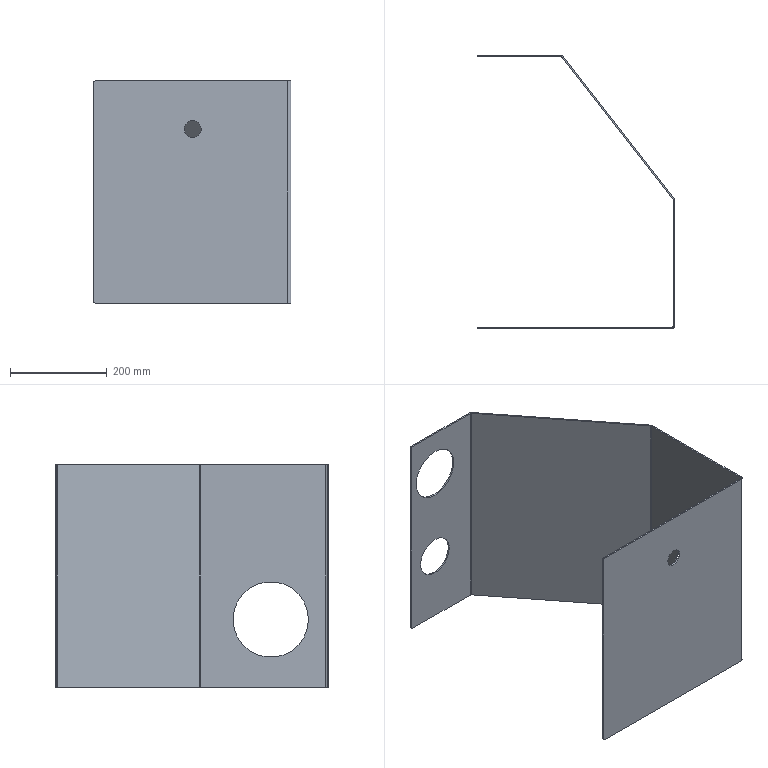Part | SolidWorks | features Cut 3, FlatPattern 1, ICE 1, SMBaseFlange 1, SheetMetal 1 | 1 solid | 42 faces | box 409 x 566 x 460 mm | volume 1582999 mm3 | plane 24 | cylinder 18 | commonest cylinder face diameters 10 x4 6 x3 12 x3 35 x2 84 x2 110 x2
STEP:
#1=CARTESIAN_POINT('',(67.,563.,305.));
#2=VERTEX_POINT('',#1);
#3=CARTESIAN_POINT('',(67.,563.,415.));
#4=VERTEX_POINT('',#3);
#5=CARTESIAN_POINT('',(67.,563.,360.));
#6=DIRECTION('',(0.,1.,0.));
#7=DIRECTION('',(0.,0.,1.));
#8=AXIS2_PLACEMENT_3D('',#5,#6,#7);
#9=CIRCLE('',#8,55.);
#10=EDGE_CURVE('',#2,#4,#9,.T.);
#11=ORIENTED_EDGE('',*,*,#10,.F.);
#12=CARTESIAN_POINT('',(67.,566.,305.));
#13=VERTEX_POINT('',#12);
#14=CARTESIAN_POINT('',(67.,563.,305.));
#15=DIRECTION('',(0.,1.,0.));
#16=VECTOR('',#15,1000.);
#17=LINE('',#14,#16);
#18=EDGE_CURVE('',#2,#13,#17,.T.);
#19=ORIENTED_EDGE('',*,*,#18,.T.);
#20=CARTESIAN_POINT('',(67.,566.,415.));
#21=VERTEX_POINT('',#20);
#22=CARTESIAN_POINT('',(67.,566.,360.));
#23=DIRECTION('',(0.,1.,0.));
#24=DIRECTION('',(0.,0.,1.));
#25=AXIS2_PLACEMENT_3D('',#22,#23,#24);
#26=CIRCLE('',#25,55.);
#27=EDGE_CURVE('',#13,#21,#26,.T.);
#28=ORIENTED_EDGE('',*,*,#27,.T.);
#29=CARTESIAN_POINT('',(67.,563.,415.));
#30=DIRECTION('',(0.,1.,0.));
#31=VECTOR('',#30,1000.);
#32=LINE('',#29,#31);
#33=EDGE_CURVE('',#4,#21,#32,.T.);
#34=ORIENTED_EDGE('',*,*,#33,.F.);
#35=EDGE_LOOP('',(#11,#19,#28,#34));
#36=FACE_OUTER_BOUND('',#35,.T.);
#37=CARTESIAN_POINT('',(67.,563.,360.));
#38=DIRECTION('',(0.,1.,0.));
#39=DIRECTION('',(0.,0.,1.));
#40=AXIS2_PLACEMENT_3D('',#37,#38,#39);
#41=CYLINDRICAL_SURFACE('',#40,55.);
#42=ADVANCED_FACE('',(#36),#41,.F.);
#43=CARTESIAN_POINT('',(67.,563.,108.));
#44=VERTEX_POINT('',#43);
#45=CARTESIAN_POINT('',(67.,563.,192.));
#46=VERTEX_POINT('',#45);
#47=CARTESIAN_POINT('',(67.,563.,150.));
#48=DIRECTION('',(0.,1.,0.));
#49=DIRECTION('',(0.,0.,1.));
#50=AXIS2_PLACEMENT_3D('',#47,#48,#49);
#51=CIRCLE('',#50,42.);
#52=EDGE_CURVE('',#44,#46,#51,.T.);
#53=ORIENTED_EDGE('',*,*,#52,.F.);
#54=CARTESIAN_POINT('',(67.,566.,108.));
#55=VERTEX_POINT('',#54);
#56=CARTESIAN_POINT('',(67.,563.,108.));
#57=DIRECTION('',(0.,1.,0.));
#58=VECTOR('',#57,1000.);
#59=LINE('',#56,#58);
#60=EDGE_CURVE('',#44,#55,#59,.T.);
#61=ORIENTED_EDGE('',*,*,#60,.T.);
#62=CARTESIAN_POINT('',(67.,566.,192.));
#63=VERTEX_POINT('',#62);
#64=CARTESIAN_POINT('',(67.,566.,150.));
#65=DIRECTION('',(0.,1.,0.));
#66=DIRECTION('',(0.,0.,1.));
#67=AXIS2_PLACEMENT_3D('',#64,#65,#66);
#68=CIRCLE('',#67,42.);
#69=EDGE_CURVE('',#55,#63,#68,.T.);
#70=ORIENTED_EDGE('',*,*,#69,.T.);
#71=CARTESIAN_POINT('',(67.,563.,192.));
#72=DIRECTION('',(0.,1.,0.));
#73=VECTOR('',#72,1000.);
#74=LINE('',#71,#73);
#75=EDGE_CURVE('',#46,#63,#74,.T.);
#76=ORIENTED_EDGE('',*,*,#75,.F.);
#77=EDGE_LOOP('',(#53,#61,#70,#76));
#78=FACE_OUTER_BOUND('',#77,.T.);
#79=CARTESIAN_POINT('',(67.,563.,150.));
#80=DIRECTION('',(0.,1.,0.));
#81=DIRECTION('',(0.,0.,1.));
#82=AXIS2_PLACEMENT_3D('',#79,#80,#81);
#83=CYLINDRICAL_SURFACE('',#82,42.);
#84=ADVANCED_FACE('',(#78),#83,.F.);
#85=CARTESIAN_POINT('',(203.,3.,377.5));
#86=VERTEX_POINT('',#85);
#87=CARTESIAN_POINT('',(203.,3.,342.5));
#88=VERTEX_POINT('',#87);
#89=CARTESIAN_POINT('',(203.,3.,360.));
#90=DIRECTION('',(0.,-1.,0.));
#91=DIRECTION('',(0.,0.,-1.));
#92=AXIS2_PLACEMENT_3D('',#89,#90,#91);
#93=CIRCLE('',#92,17.5);
#94=EDGE_CURVE('',#86,#88,#93,.T.);
#95=ORIENTED_EDGE('',*,*,#94,.F.);
#96=CARTESIAN_POINT('',(203.,0.,377.5));
#97=VERTEX_POINT('',#96);
#98=CARTESIAN_POINT('',(203.,3.,377.5));
#99=DIRECTION('',(0.,-1.,0.));
#100=VECTOR('',#99,1000.);
#101=LINE('',#98,#100);
#102=EDGE_CURVE('',#86,#97,#101,.T.);
#103=ORIENTED_EDGE('',*,*,#102,.T.);
#104=CARTESIAN_POINT('',(203.,0.,342.5));
#105=VERTEX_POINT('',#104);
#106=CARTESIAN_POINT('',(203.,0.,360.));
#107=DIRECTION('',(0.,-1.,0.));
#108=DIRECTION('',(0.,0.,-1.));
#109=AXIS2_PLACEMENT_3D('',#106,#107,#108);
#110=CIRCLE('',#109,17.5);
#111=EDGE_CURVE('',#97,#105,#110,.T.);
#112=ORIENTED_EDGE('',*,*,#111,.T.);
#113=CARTESIAN_POINT('',(203.,3.,342.5));
#114=DIRECTION('',(0.,-1.,0.));
#115=VECTOR('',#114,1000.);
#116=LINE('',#113,#115);
#117=EDGE_CURVE('',#88,#105,#116,.T.);
#118=ORIENTED_EDGE('',*,*,#117,.F.);
#119=EDGE_LOOP('',(#95,#103,#112,#118));
#120=FACE_OUTER_BOUND('',#119,.T.);
#121=CARTESIAN_POINT('',(203.,3.,360.));
#122=DIRECTION('',(0.,-1.,0.));
#123=DIRECTION('',(0.,0.,-1.));
#124=AXIS2_PLACEMENT_3D('',#121,#122,#123);
#125=CYLINDRICAL_SURFACE('',#124,17.5);
#126=ADVANCED_FACE('',(#120),#125,.F.);
#127=CARTESIAN_POINT('',(403.,42.,140.));
#128=VERTEX_POINT('',#127);
#129=CARTESIAN_POINT('',(403.,198.,140.));
#130=VERTEX_POINT('',#129);
#131=CARTESIAN_POINT('',(403.,120.,140.));
#132=DIRECTION('',(1.,0.,0.));
#133=DIRECTION('',(0.,1.,0.));
#134=AXIS2_PLACEMENT_3D('',#131,#132,#133);
#135=CIRCLE('',#134,78.);
#136=EDGE_CURVE('',#128,#130,#135,.T.);
#137=ORIENTED_EDGE('',*,*,#136,.F.);
#138=CARTESIAN_POINT('',(406.,42.,140.));
#139=VERTEX_POINT('',#138);
#140=CARTESIAN_POINT('',(396.,42.,140.));
#141=DIRECTION('',(1.,0.,0.));
#142=VECTOR('',#141,1000.);
#143=LINE('',#140,#142);
#144=EDGE_CURVE('',#128,#139,#143,.T.);
#145=ORIENTED_EDGE('',*,*,#144,.T.);
#146=CARTESIAN_POINT('',(406.,198.,140.));
#147=VERTEX_POINT('',#146);
#148=CARTESIAN_POINT('',(406.,120.,140.));
#149=DIRECTION('',(1.,0.,0.));
#150=DIRECTION('',(0.,1.,0.));
#151=AXIS2_PLACEMENT_3D('',#148,#149,#150);
#152=CIRCLE('',#151,78.);
#153=EDGE_CURVE('',#139,#147,#152,.T.);
#154=ORIENTED_EDGE('',*,*,#153,.T.);
#155=CARTESIAN_POINT('',(396.,198.,140.));
#156=DIRECTION('',(1.,0.,0.));
#157=VECTOR('',#156,1000.);
#158=LINE('',#155,#157);
#159=EDGE_CURVE('',#130,#147,#158,.T.);
#160=ORIENTED_EDGE('',*,*,#159,.F.);
#161=EDGE_LOOP('',(#137,#145,#154,#160));
#162=FACE_OUTER_BOUND('',#161,.T.);
#163=CARTESIAN_POINT('',(396.,120.,140.));
#164=DIRECTION('',(1.,0.,0.));
#165=DIRECTION('',(0.,1.,0.));
#166=AXIS2_PLACEMENT_3D('',#163,#164,#165);
#167=CYLINDRICAL_SURFACE('',#166,78.);
#168=ADVANCED_FACE('',(#162),#167,.F.);
#169=CARTESIAN_POINT('',(67.,566.,360.));
#170=DIRECTION('',(0.,1.,0.));
#171=DIRECTION('',(0.,0.,1.));
#172=AXIS2_PLACEMENT_3D('',#169,#170,#171);
#173=CIRCLE('',#172,55.);
#174=EDGE_CURVE('',#21,#13,#173,.T.);
#175=ORIENTED_EDGE('',*,*,#174,.F.);
#176=ORIENTED_EDGE('',*,*,#27,.F.);
#177=EDGE_LOOP('',(#175,#176));
#178=FACE_BOUND('',#177,.T.);
#179=CARTESIAN_POINT('',(67.,566.,150.));
#180=DIRECTION('',(0.,1.,0.));
#181=DIRECTION('',(0.,0.,1.));
#182=AXIS2_PLACEMENT_3D('',#179,#180,#181);
#183=CIRCLE('',#182,42.);
#184=EDGE_CURVE('',#63,#55,#183,.T.);
#185=ORIENTED_EDGE('',*,*,#184,.F.);
#186=ORIENTED_EDGE('',*,*,#69,.F.);
#187=EDGE_LOOP('',(#185,#186));
#188=FACE_BOUND('',#187,.T.);
#189=CARTESIAN_POINT('',(2.,566.,0.));
#190=VERTEX_POINT('',#189);
#191=CARTESIAN_POINT('',(170.25,566.,0.));
#192=VERTEX_POINT('',#191);
#193=CARTESIAN_POINT('',(-3.,566.,0.));
#194=DIRECTION('',(1.,0.,0.));
#195=VECTOR('',#194,1000.);
#196=LINE('',#193,#195);
#197=EDGE_CURVE('',#190,#192,#196,.T.);
#198=ORIENTED_EDGE('',*,*,#197,.F.);
#199=CARTESIAN_POINT('',(-3.,566.,5.));
#200=VERTEX_POINT('',#199);
#201=CARTESIAN_POINT('',(2.,566.,5.));
#202=DIRECTION('',(0.,-1.,0.));
#203=DIRECTION('',(0.,0.,1.));
#204=AXIS2_PLACEMENT_3D('',#201,#202,#203);
#205=CIRCLE('',#204,5.);
#206=EDGE_CURVE('',#200,#190,#205,.T.);
#207=ORIENTED_EDGE('',*,*,#206,.F.);
#208=CARTESIAN_POINT('',(-3.,566.,455.));
#209=VERTEX_POINT('',#208);
#210=CARTESIAN_POINT('',(-3.,566.,460.));
#211=DIRECTION('',(0.,0.,-1.));
#212=VECTOR('',#211,1000.);
#213=LINE('',#210,#212);
#214=EDGE_CURVE('',#209,#200,#213,.T.);
#215=ORIENTED_EDGE('',*,*,#214,.F.);
#216=CARTESIAN_POINT('',(2.,566.,460.));
#217=VERTEX_POINT('',#216);
#218=CARTESIAN_POINT('',(2.,566.,455.));
#219=DIRECTION('',(0.,-1.,0.));
#220=DIRECTION('',(0.,0.,1.));
#221=AXIS2_PLACEMENT_3D('',#218,#219,#220);
#222=CIRCLE('',#221,5.);
#223=EDGE_CURVE('',#217,#209,#222,.T.);
#224=ORIENTED_EDGE('',*,*,#223,.F.);
#225=CARTESIAN_POINT('',(170.25,566.,460.));
#226=VERTEX_POINT('',#225);
#227=CARTESIAN_POINT('',(-3.,566.,460.));
#228=DIRECTION('',(1.,0.,0.));
#229=VECTOR('',#228,1000.);
#230=LINE('',#227,#229);
#231=EDGE_CURVE('',#217,#226,#230,.T.);
#232=ORIENTED_EDGE('',*,*,#231,.T.);
#233=CARTESIAN_POINT('',(170.25,566.,460.));
#234=DIRECTION('',(0.,0.,-1.));
#235=VECTOR('',#234,1000.);
#236=LINE('',#233,#235);
#237=EDGE_CURVE('',#226,#192,#236,.T.);
#238=ORIENTED_EDGE('',*,*,#237,.T.);
#239=EDGE_LOOP('',(#198,#207,#215,#224,#232,#238));
#240=FACE_OUTER_BOUND('',#239,.T.);
#241=CARTESIAN_POINT('',(-3.,566.,460.));
#242=DIRECTION('',(0.,1.,0.));
#243=DIRECTION('',(0.,0.,1.));
#244=AXIS2_PLACEMENT_3D('',#241,#242,#243);
#245=PLANE('',#244);
#246=ADVANCED_FACE('',(#178,#188,#240),#245,.T.);
#247=CARTESIAN_POINT('',(67.,563.,360.));
#248=DIRECTION('',(0.,1.,0.));
#249=DIRECTION('',(0.,0.,1.));
#250=AXIS2_PLACEMENT_3D('',#247,#248,#249);
#251=CIRCLE('',#250,55.);
#252=EDGE_CURVE('',#4,#2,#251,.T.);
#253=ORIENTED_EDGE('',*,*,#252,.T.);
#254=ORIENTED_EDGE('',*,*,#10,.T.);
#255=EDGE_LOOP('',(#253,#254));
#256=FACE_BOUND('',#255,.T.);
#257=CARTESIAN_POINT('',(67.,563.,150.));
#258=DIRECTION('',(0.,1.,0.));
#259=DIRECTION('',(0.,0.,1.));
#260=AXIS2_PLACEMENT_3D('',#257,#258,#259);
#261=CIRCLE('',#260,42.);
#262=EDGE_CURVE('',#46,#44,#261,.T.);
#263=ORIENTED_EDGE('',*,*,#262,.T.);
#264=ORIENTED_EDGE('',*,*,#52,.T.);
#265=EDGE_LOOP('',(#263,#264));
#266=FACE_BOUND('',#265,.T.);
#267=CARTESIAN_POINT('',(-3.,563.,5.));
#268=VERTEX_POINT('',#267);
#269=CARTESIAN_POINT('',(2.,563.,0.));
#270=VERTEX_POINT('',#269);
#271=CARTESIAN_POINT('',(2.,563.,5.));
#272=DIRECTION('',(0.,-1.,0.));
#273=DIRECTION('',(0.,0.,1.));
#274=AXIS2_PLACEMENT_3D('',#271,#272,#273);
#275=CIRCLE('',#274,5.);
#276=EDGE_CURVE('',#268,#270,#275,.T.);
#277=ORIENTED_EDGE('',*,*,#276,.T.);
#278=CARTESIAN_POINT('',(170.25,563.,0.));
#279=VERTEX_POINT('',#278);
#280=CARTESIAN_POINT('',(-3.,563.,0.));
#281=DIRECTION('',(1.,0.,0.));
#282=VECTOR('',#281,1000.);
#283=LINE('',#280,#282);
#284=EDGE_CURVE('',#270,#279,#283,.T.);
#285=ORIENTED_EDGE('',*,*,#284,.T.);
#286=CARTESIAN_POINT('',(170.25,563.,460.));
#287=VERTEX_POINT('',#286);
#288=CARTESIAN_POINT('',(170.25,563.,460.));
#289=DIRECTION('',(0.,0.,-1.));
#290=VECTOR('',#289,1000.);
#291=LINE('',#288,#290);
#292=EDGE_CURVE('',#287,#279,#291,.T.);
#293=ORIENTED_EDGE('',*,*,#292,.F.);
#294=CARTESIAN_POINT('',(2.,563.,460.));
#295=VERTEX_POINT('',#294);
#296=CARTESIAN_POINT('',(-3.,563.,460.));
#297=DIRECTION('',(1.,0.,0.));
#298=VECTOR('',#297,1000.);
#299=LINE('',#296,#298);
#300=EDGE_CURVE('',#295,#287,#299,.T.);
#301=ORIENTED_EDGE('',*,*,#300,.F.);
#302=CARTESIAN_POINT('',(-3.,563.,455.));
#303=VERTEX_POINT('',#302);
#304=CARTESIAN_POINT('',(2.,563.,455.));
#305=DIRECTION('',(0.,-1.,0.));
#306=DIRECTION('',(0.,0.,1.));
#307=AXIS2_PLACEMENT_3D('',#304,#305,#306);
#308=CIRCLE('',#307,5.);
#309=EDGE_CURVE('',#295,#303,#308,.T.);
#310=ORIENTED_EDGE('',*,*,#309,.T.);
#311=CARTESIAN_POINT('',(-3.,563.,460.));
#312=DIRECTION('',(0.,0.,-1.));
#313=VECTOR('',#312,1000.);
#314=LINE('',#311,#313);
#315=EDGE_CURVE('',#303,#268,#314,.T.);
#316=ORIENTED_EDGE('',*,*,#315,.T.);
#317=EDGE_LOOP('',(#277,#285,#293,#301,#310,#316));
#318=FACE_OUTER_BOUND('',#317,.T.);
#319=CARTESIAN_POINT('',(-3.,563.,460.));
#320=DIRECTION('',(0.,1.,0.));
#321=DIRECTION('',(0.,0.,1.));
#322=AXIS2_PLACEMENT_3D('',#319,#320,#321);
#323=PLANE('',#322);
#324=ADVANCED_FACE('',(#256,#266,#318),#323,.F.);
#325=ORIENTED_EDGE('',*,*,#284,.F.);
#326=CARTESIAN_POINT('',(2.,563.,0.));
#327=DIRECTION('',(0.,1.,0.));
#328=VECTOR('',#327,1000.);
#329=LINE('',#326,#328);
#330=EDGE_CURVE('',#270,#190,#329,.T.);
#331=ORIENTED_EDGE('',*,*,#330,.T.);
#332=ORIENTED_EDGE('',*,*,#197,.T.);
#333=CARTESIAN_POINT('',(170.25,566.,0.));
#334=DIRECTION('',(0.,-1.,0.));
#335=VECTOR('',#334,1000.);
#336=LINE('',#333,#335);
#337=EDGE_CURVE('',#192,#279,#336,.T.);
#338=ORIENTED_EDGE('',*,*,#337,.T.);
#339=EDGE_LOOP('',(#325,#331,#332,#338));
#340=FACE_OUTER_BOUND('',#339,.T.);
#341=CARTESIAN_POINT('',(172.615,561.847,0.));
#342=DIRECTION('',(0.,0.,-1.));
#343=DIRECTION('',(-1.,0.,0.));
#344=AXIS2_PLACEMENT_3D('',#341,#342,#343);
#345=PLANE('',#344);
#346=ADVANCED_FACE('',(#340),#345,.T.);
#347=CARTESIAN_POINT('',(203.,0.,360.));
#348=DIRECTION('',(0.,-1.,0.));
#349=DIRECTION('',(0.,0.,-1.));
#350=AXIS2_PLACEMENT_3D('',#347,#348,#349);
#351=CIRCLE('',#350,17.5);
#352=EDGE_CURVE('',#105,#97,#351,.T.);
#353=ORIENTED_EDGE('',*,*,#352,.F.);
#354=ORIENTED_EDGE('',*,*,#111,.F.);
#355=EDGE_LOOP('',(#353,#354));
#356=FACE_BOUND('',#355,.T.);
#357=CARTESIAN_POINT('',(-3.,0.,455.));
#358=VERTEX_POINT('',#357);
#359=CARTESIAN_POINT('',(-3.,0.,5.));
#360=VERTEX_POINT('',#359);
#361=CARTESIAN_POINT('',(-3.,0.,460.));
#362=DIRECTION('',(0.,0.,-1.));
#363=VECTOR('',#362,1000.);
#364=LINE('',#361,#363);
#365=EDGE_CURVE('',#358,#360,#364,.T.);
#366=ORIENTED_EDGE('',*,*,#365,.T.);
#367=CARTESIAN_POINT('',(2.,0.,0.));
#368=VERTEX_POINT('',#367);
#369=CARTESIAN_POINT('',(2.,0.,5.));
#370=DIRECTION('',(0.,1.,0.));
#371=DIRECTION('',(0.,0.,-1.));
#372=AXIS2_PLACEMENT_3D('',#369,#370,#371);
#373=CIRCLE('',#372,5.);
#374=EDGE_CURVE('',#368,#360,#373,.T.);
#375=ORIENTED_EDGE('',*,*,#374,.F.);
#376=CARTESIAN_POINT('',(400.,0.,0.));
#377=VERTEX_POINT('',#376);
#378=CARTESIAN_POINT('',(0.,0.,0.));
#379=DIRECTION('',(-1.,0.,0.));
#380=VECTOR('',#379,1000.);
#381=LINE('',#378,#380);
#382=EDGE_CURVE('',#377,#368,#381,.T.);
#383=ORIENTED_EDGE('',*,*,#382,.F.);
#384=CARTESIAN_POINT('',(400.,0.,460.));
#385=VERTEX_POINT('',#384);
#386=CARTESIAN_POINT('',(400.,0.,460.));
#387=DIRECTION('',(0.,0.,-1.));
#388=VECTOR('',#387,1000.);
#389=LINE('',#386,#388);
#390=EDGE_CURVE('',#385,#377,#389,.T.);
#391=ORIENTED_EDGE('',*,*,#390,.F.);
#392=CARTESIAN_POINT('',(2.,0.,460.));
#393=VERTEX_POINT('',#392);
#394=CARTESIAN_POINT('',(0.,0.,460.));
#395=DIRECTION('',(-1.,0.,0.));
#396=VECTOR('',#395,1000.);
#397=LINE('',#394,#396);
#398=EDGE_CURVE('',#385,#393,#397,.T.);
#399=ORIENTED_EDGE('',*,*,#398,.T.);
#400=CARTESIAN_POINT('',(2.,0.,455.));
#401=DIRECTION('',(0.,1.,0.));
#402=DIRECTION('',(0.,0.,-1.));
#403=AXIS2_PLACEMENT_3D('',#400,#401,#402);
#404=CIRCLE('',#403,5.);
#405=EDGE_CURVE('',#358,#393,#404,.T.);
#406=ORIENTED_EDGE('',*,*,#405,.F.);
#407=EDGE_LOOP('',(#366,#375,#383,#391,#399,#406));
#408=FACE_OUTER_BOUND('',#407,.T.);
#409=CARTESIAN_POINT('',(0.,0.,460.));
#410=DIRECTION('',(0.,-1.,0.));
#411=DIRECTION('',(0.,0.,-1.));
#412=AXIS2_PLACEMENT_3D('',#409,#410,#411);
#413=PLANE('',#412);
#414=ADVANCED_FACE('',(#356,#408),#413,.T.);
#415=CARTESIAN_POINT('',(203.,3.,360.));
#416=DIRECTION('',(0.,-1.,0.));
#417=DIRECTION('',(0.,0.,-1.));
#418=AXIS2_PLACEMENT_3D('',#415,#416,#417);
#419=CIRCLE('',#418,17.5);
#420=EDGE_CURVE('',#88,#86,#419,.T.);
#421=ORIENTED_EDGE('',*,*,#420,.T.);
#422=ORIENTED_EDGE('',*,*,#94,.T.);
#423=EDGE_LOOP('',(#421,#422));
#424=FACE_BOUND('',#423,.T.);
#425=CARTESIAN_POINT('',(2.,3.,0.));
#426=VERTEX_POINT('',#425);
#427=CARTESIAN_POINT('',(-3.,3.,5.));
#428=VERTEX_POINT('',#427);
#429=CARTESIAN_POINT('',(2.,3.,5.));
#430=DIRECTION('',(0.,1.,0.));
#431=DIRECTION('',(0.,0.,-1.));
#432=AXIS2_PLACEMENT_3D('',#429,#430,#431);
#433=CIRCLE('',#432,5.);
#434=EDGE_CURVE('',#426,#428,#433,.T.);
#435=ORIENTED_EDGE('',*,*,#434,.T.);
#436=CARTESIAN_POINT('',(-3.,3.,455.));
#437=VERTEX_POINT('',#436);
#438=CARTESIAN_POINT('',(-3.,3.,460.));
#439=DIRECTION('',(0.,0.,-1.));
#440=VECTOR('',#439,1000.);
#441=LINE('',#438,#440);
#442=EDGE_CURVE('',#437,#428,#441,.T.);
#443=ORIENTED_EDGE('',*,*,#442,.F.);
#444=CARTESIAN_POINT('',(2.,3.,460.));
#445=VERTEX_POINT('',#444);
#446=CARTESIAN_POINT('',(2.,3.,455.));
#447=DIRECTION('',(0.,1.,0.));
#448=DIRECTION('',(0.,0.,-1.));
#449=AXIS2_PLACEMENT_3D('',#446,#447,#448);
#450=CIRCLE('',#449,5.);
#451=EDGE_CURVE('',#437,#445,#450,.T.);
#452=ORIENTED_EDGE('',*,*,#451,.T.);
#453=CARTESIAN_POINT('',(400.,3.,460.));
#454=VERTEX_POINT('',#453);
#455=CARTESIAN_POINT('',(0.,3.,460.));
#456=DIRECTION('',(-1.,0.,0.));
#457=VECTOR('',#456,1000.);
#458=LINE('',#455,#457);
#459=EDGE_CURVE('',#454,#445,#458,.T.);
#460=ORIENTED_EDGE('',*,*,#459,.F.);
#461=CARTESIAN_POINT('',(400.,3.,0.));
#462=VERTEX_POINT('',#461);
#463=CARTESIAN_POINT('',(400.,3.,460.));
#464=DIRECTION('',(0.,0.,-1.));
#465=VECTOR('',#464,1000.);
#466=LINE('',#463,#465);
#467=EDGE_CURVE('',#454,#462,#466,.T.);
#468=ORIENTED_EDGE('',*,*,#467,.T.);
#469=CARTESIAN_POINT('',(0.,3.,0.));
#470=DIRECTION('',(-1.,0.,0.));
#471=VECTOR('',#470,1000.);
#472=LINE('',#469,#471);
#473=EDGE_CURVE('',#462,#426,#472,.T.);
#474=ORIENTED_EDGE('',*,*,#473,.T.);
#475=EDGE_LOOP('',(#435,#443,#452,#460,#468,#474));
#476=FACE_OUTER_BOUND('',#475,.T.);
#477=CARTESIAN_POINT('',(0.,3.,460.));
#478=DIRECTION('',(0.,-1.,0.));
#479=DIRECTION('',(0.,0.,-1.));
#480=AXIS2_PLACEMENT_3D('',#477,#478,#479);
#481=PLANE('',#480);
#482=ADVANCED_FACE('',(#424,#476),#481,.F.);
#483=ORIENTED_EDGE('',*,*,#442,.T.);
#484=CARTESIAN_POINT('',(-3.,3.,5.));
#485=DIRECTION('',(0.,-1.,0.));
#486=VECTOR('',#485,1000.);
#487=LINE('',#484,#486);
#488=EDGE_CURVE('',#428,#360,#487,.T.);
#489=ORIENTED_EDGE('',*,*,#488,.T.);
#490=ORIENTED_EDGE('',*,*,#365,.F.);
#491=CARTESIAN_POINT('',(-3.,3.,455.));
#492=DIRECTION('',(0.,-1.,0.));
#493=VECTOR('',#492,1000.);
#494=LINE('',#491,#493);
#495=EDGE_CURVE('',#437,#358,#494,.T.);
#496=ORIENTED_EDGE('',*,*,#495,.F.);
#497=EDGE_LOOP('',(#483,#489,#490,#496));
#498=FACE_OUTER_BOUND('',#497,.T.);
#499=CARTESIAN_POINT('',(-3.,0.,460.));
#500=DIRECTION('',(-1.,0.,0.));
#501=DIRECTION('',(0.,-1.,0.));
#502=AXIS2_PLACEMENT_3D('',#499,#500,#501);
#503=PLANE('',#502);
#504=ADVANCED_FACE('',(#498),#503,.T.);
#505=CARTESIAN_POINT('',(-3.,563.,5.));
#506=DIRECTION('',(0.,1.,0.));
#507=VECTOR('',#506,1000.);
#508=LINE('',#505,#507);
#509=EDGE_CURVE('',#268,#200,#508,.T.);
#510=ORIENTED_EDGE('',*,*,#509,.F.);
#511=ORIENTED_EDGE('',*,*,#315,.F.);
#512=CARTESIAN_POINT('',(-3.,563.,455.));
#513=DIRECTION('',(0.,1.,0.));
#514=VECTOR('',#513,1000.);
#515=LINE('',#512,#514);
#516=EDGE_CURVE('',#303,#209,#515,.T.);
#517=ORIENTED_EDGE('',*,*,#516,.T.);
#518=ORIENTED_EDGE('',*,*,#214,.T.);
#519=EDGE_LOOP('',(#510,#511,#517,#518));
#520=FACE_OUTER_BOUND('',#519,.T.);
#521=CARTESIAN_POINT('',(-3.,563.,460.));
#522=DIRECTION('',(-1.,0.,0.));
#523=DIRECTION('',(0.,0.,1.));
#524=AXIS2_PLACEMENT_3D('',#521,#522,#523);
#525=PLANE('',#524);
#526=ADVANCED_FACE('',(#520),#525,.T.);
#527=CARTESIAN_POINT('',(2.,563.,460.));
#528=DIRECTION('',(0.,1.,0.));
#529=VECTOR('',#528,1000.);
#530=LINE('',#527,#529);
#531=EDGE_CURVE('',#295,#217,#530,.T.);
#532=ORIENTED_EDGE('',*,*,#531,.F.);
#533=ORIENTED_EDGE('',*,*,#300,.T.);
#534=CARTESIAN_POINT('',(170.25,563.,460.));
#535=DIRECTION('',(0.,1.,0.));
#536=VECTOR('',#535,1000.);
#537=LINE('',#534,#536);
#538=EDGE_CURVE('',#287,#226,#537,.T.);
#539=ORIENTED_EDGE('',*,*,#538,.T.);
#540=ORIENTED_EDGE('',*,*,#231,.F.);
#541=EDGE_LOOP('',(#532,#533,#539,#540));
#542=FACE_OUTER_BOUND('',#541,.T.);
#543=CARTESIAN_POINT('',(400.,6.,460.));
#544=DIRECTION('',(0.,0.,-1.));
#545=DIRECTION('',(-1.,0.,0.));
#546=AXIS2_PLACEMENT_3D('',#543,#544,#545);
#547=PLANE('',#546);
#548=ADVANCED_FACE('',(#542),#547,.F.);
#549=ORIENTED_EDGE('',*,*,#459,.T.);
#550=CARTESIAN_POINT('',(2.,3.,460.));
#551=DIRECTION('',(0.,-1.,0.));
#552=VECTOR('',#551,1000.);
#553=LINE('',#550,#552);
#554=EDGE_CURVE('',#445,#393,#553,.T.);
#555=ORIENTED_EDGE('',*,*,#554,.T.);
#556=ORIENTED_EDGE('',*,*,#398,.F.);
#557=CARTESIAN_POINT('',(400.,0.,460.));
#558=DIRECTION('',(0.,1.,0.));
#559=VECTOR('',#558,1000.);
#560=LINE('',#557,#559);
#561=EDGE_CURVE('',#385,#454,#560,.T.);
#562=ORIENTED_EDGE('',*,*,#561,.T.);
#563=EDGE_LOOP('',(#549,#555,#556,#562));
#564=FACE_OUTER_BOUND('',#563,.T.);
#565=CARTESIAN_POINT('',(403.,6.,460.));
#566=DIRECTION('',(0.,0.,1.));
#567=DIRECTION('',(1.,0.,0.));
#568=AXIS2_PLACEMENT_3D('',#565,#566,#567);
#569=PLANE('',#568);
#570=ADVANCED_FACE('',(#564),#569,.T.);
#571=ORIENTED_EDGE('',*,*,#561,.F.);
#572=CARTESIAN_POINT('',(406.,6.,460.));
#573=VERTEX_POINT('',#572);
#574=CARTESIAN_POINT('',(400.,6.,460.));
#575=DIRECTION('',(0.,0.,-1.));
#576=DIRECTION('',(-1.,0.,0.));
#577=AXIS2_PLACEMENT_3D('',#574,#575,#576);
#578=CIRCLE('',#577,6.);
#579=EDGE_CURVE('',#573,#385,#578,.T.);
#580=ORIENTED_EDGE('',*,*,#579,.F.);
#581=CARTESIAN_POINT('',(403.,6.,460.));
#582=VERTEX_POINT('',#581);
#583=CARTESIAN_POINT('',(403.,6.,460.));
#584=DIRECTION('',(1.,0.,0.));
#585=VECTOR('',#584,1000.);
#586=LINE('',#583,#585);
#587=EDGE_CURVE('',#582,#573,#586,.T.);
#588=ORIENTED_EDGE('',*,*,#587,.F.);
#589=CARTESIAN_POINT('',(400.,6.,460.));
#590=DIRECTION('',(0.,0.,-1.));
#591=DIRECTION('',(1.,0.,0.));
#592=AXIS2_PLACEMENT_3D('',#589,#590,#591);
#593=CIRCLE('',#592,3.);
#594=EDGE_CURVE('',#582,#454,#593,.T.);
#595=ORIENTED_EDGE('',*,*,#594,.T.);
#596=EDGE_LOOP('',(#571,#580,#588,#595));
#597=FACE_OUTER_BOUND('',#596,.T.);
#598=CARTESIAN_POINT('',(400.,0.,460.));
#599=DIRECTION('',(0.,0.,1.));
#600=DIRECTION('',(1.,0.,0.));
#601=AXIS2_PLACEMENT_3D('',#598,#599,#600);
#602=PLANE('',#601);
#603=ADVANCED_FACE('',(#597),#602,.T.);
#604=CARTESIAN_POINT('',(406.,6.,0.));
#605=VERTEX_POINT('',#604);
#606=CARTESIAN_POINT('',(403.,6.,0.));
#607=VERTEX_POINT('',#606);
#608=CARTESIAN_POINT('',(406.,6.,0.));
#609=DIRECTION('',(-1.,0.,0.));
#610=VECTOR('',#609,1000.);
#611=LINE('',#608,#610);
#612=EDGE_CURVE('',#605,#607,#611,.T.);
#613=ORIENTED_EDGE('',*,*,#612,.F.);
#614=CARTESIAN_POINT('',(400.,6.,0.));
#615=DIRECTION('',(0.,0.,-1.));
#616=DIRECTION('',(-1.,0.,0.));
#617=AXIS2_PLACEMENT_3D('',#614,#615,#616);
#618=CIRCLE('',#617,6.);
#619=EDGE_CURVE('',#605,#377,#618,.T.);
#620=ORIENTED_EDGE('',*,*,#619,.T.);
#621=CARTESIAN_POINT('',(400.,3.,0.));
#622=DIRECTION('',(0.,-1.,0.));
#623=VECTOR('',#622,1000.);
#624=LINE('',#621,#623);
#625=EDGE_CURVE('',#462,#377,#624,.T.);
#626=ORIENTED_EDGE('',*,*,#625,.F.);
#627=CARTESIAN_POINT('',(400.,6.,0.));
#628=DIRECTION('',(0.,0.,-1.));
#629=DIRECTION('',(1.,0.,0.));
#630=AXIS2_PLACEMENT_3D('',#627,#628,#629);
#631=CIRCLE('',#630,3.);
#632=EDGE_CURVE('',#607,#462,#631,.T.);
#633=ORIENTED_EDGE('',*,*,#632,.F.);
#634=EDGE_LOOP('',(#613,#620,#626,#633));
#635=FACE_OUTER_BOUND('',#634,.T.);
#636=CARTESIAN_POINT('',(406.,6.,0.));
#637=DIRECTION('',(0.,0.,-1.));
#638=DIRECTION('',(-1.,0.,0.));
#639=AXIS2_PLACEMENT_3D('',#636,#637,#638);
#640=PLANE('',#639);
#641=ADVANCED_FACE('',(#635),#640,.T.);
#642=CARTESIAN_POINT('',(406.,265.934,0.));
#643=VERTEX_POINT('',#642);
#644=CARTESIAN_POINT('',(406.,0.,0.));
#645=DIRECTION('',(0.,-1.,0.));
#646=VECTOR('',#645,1000.);
#647=LINE('',#644,#646);
#648=EDGE_CURVE('',#643,#605,#647,.T.);
#649=ORIENTED_EDGE('',*,*,#648,.T.);
#650=ORIENTED_EDGE('',*,*,#612,.T.);
#651=CARTESIAN_POINT('',(403.,265.934,0.));
#652=VERTEX_POINT('',#651);
#653=CARTESIAN_POINT('',(403.,0.,0.));
#654=DIRECTION('',(0.,-1.,0.));
#655=VECTOR('',#654,1000.);
#656=LINE('',#653,#655);
#657=EDGE_CURVE('',#652,#607,#656,.T.);
#658=ORIENTED_EDGE('',*,*,#657,.F.);
#659=CARTESIAN_POINT('',(403.,265.934,0.));
#660=DIRECTION('',(1.,0.,0.));
#661=VECTOR('',#660,1000.);
#662=LINE('',#659,#661);
#663=EDGE_CURVE('',#652,#643,#662,.T.);
#664=ORIENTED_EDGE('',*,*,#663,.T.);
#665=EDGE_LOOP('',(#649,#650,#658,#664));
#666=FACE_OUTER_BOUND('',#665,.T.);
#667=CARTESIAN_POINT('',(400.,3.,0.));
#668=DIRECTION('',(0.,0.,-1.));
#669=DIRECTION('',(-1.,0.,0.));
#670=AXIS2_PLACEMENT_3D('',#667,#668,#669);
#671=PLANE('',#670);
#672=ADVANCED_FACE('',(#666),#671,.T.);
#673=CARTESIAN_POINT('',(406.,265.934,460.));
#674=VERTEX_POINT('',#673);
#675=CARTESIAN_POINT('',(403.,265.934,460.));
#676=VERTEX_POINT('',#675);
#677=CARTESIAN_POINT('',(406.,265.934,460.));
#678=DIRECTION('',(-1.,0.,0.));
#679=VECTOR('',#678,1000.);
#680=LINE('',#677,#679);
#681=EDGE_CURVE('',#674,#676,#680,.T.);
#682=ORIENTED_EDGE('',*,*,#681,.F.);
#683=CARTESIAN_POINT('',(404.728,269.628,460.));
#684=VERTEX_POINT('',#683);
#685=CARTESIAN_POINT('',(400.,265.934,460.));
#686=DIRECTION('',(0.,0.,-1.));
#687=DIRECTION('',(-1.,0.,0.));
#688=AXIS2_PLACEMENT_3D('',#685,#686,#687);
#689=CIRCLE('',#688,6.);
#690=EDGE_CURVE('',#684,#674,#689,.T.);
#691=ORIENTED_EDGE('',*,*,#690,.F.);
#692=CARTESIAN_POINT('',(402.364,267.781,460.));
#693=VERTEX_POINT('',#692);
#694=CARTESIAN_POINT('',(402.364,267.781,460.));
#695=DIRECTION('',(0.788,0.6157,0.));
#696=VECTOR('',#695,1000.);
#697=LINE('',#694,#696);
#698=EDGE_CURVE('',#693,#684,#697,.T.);
#699=ORIENTED_EDGE('',*,*,#698,.F.);
#700=CARTESIAN_POINT('',(400.,265.934,460.));
#701=DIRECTION('',(0.,0.,-1.));
#702=DIRECTION('',(1.,0.,0.));
#703=AXIS2_PLACEMENT_3D('',#700,#701,#702);
#704=CIRCLE('',#703,3.);
#705=EDGE_CURVE('',#693,#676,#704,.T.);
#706=ORIENTED_EDGE('',*,*,#705,.T.);
#707=EDGE_LOOP('',(#682,#691,#699,#706));
#708=FACE_OUTER_BOUND('',#707,.T.);
#709=CARTESIAN_POINT('',(406.,265.934,460.));
#710=DIRECTION('',(0.,0.,1.));
#711=DIRECTION('',(1.,0.,0.));
#712=AXIS2_PLACEMENT_3D('',#709,#710,#711);
#713=PLANE('',#712);
#714=ADVANCED_FACE('',(#708),#713,.T.);
#715=CARTESIAN_POINT('',(406.,0.,460.));
#716=DIRECTION('',(0.,-1.,0.));
#717=VECTOR('',#716,1000.);
#718=LINE('',#715,#717);
#719=EDGE_CURVE('',#674,#573,#718,.T.);
#720=ORIENTED_EDGE('',*,*,#719,.F.);
#721=ORIENTED_EDGE('',*,*,#681,.T.);
#722=CARTESIAN_POINT('',(403.,0.,460.));
#723=DIRECTION('',(0.,-1.,0.));
#724=VECTOR('',#723,1000.);
#725=LINE('',#722,#724);
#726=EDGE_CURVE('',#676,#582,#725,.T.);
#727=ORIENTED_EDGE('',*,*,#726,.T.);
#728=ORIENTED_EDGE('',*,*,#587,.T.);
#729=EDGE_LOOP('',(#720,#721,#727,#728));
#730=FACE_OUTER_BOUND('',#729,.T.);
#731=CARTESIAN_POINT('',(402.364,267.781,460.));
#732=DIRECTION('',(0.,0.,1.));
#733=DIRECTION('',(1.,0.,0.));
#734=AXIS2_PLACEMENT_3D('',#731,#732,#733);
#735=PLANE('',#734);
#736=ADVANCED_FACE('',(#730),#735,.T.);
#737=CARTESIAN_POINT('',(404.728,269.628,0.));
#738=VERTEX_POINT('',#737);
#739=CARTESIAN_POINT('',(402.364,267.781,0.));
#740=VERTEX_POINT('',#739);
#741=CARTESIAN_POINT('',(404.728,269.628,0.));
#742=DIRECTION('',(-0.788,-0.6157,0.));
#743=VECTOR('',#742,1000.);
#744=LINE('',#741,#743);
#745=EDGE_CURVE('',#738,#740,#744,.T.);
#746=ORIENTED_EDGE('',*,*,#745,.F.);
#747=CARTESIAN_POINT('',(400.,265.934,0.));
#748=DIRECTION('',(0.,0.,-1.));
#749=DIRECTION('',(-1.,0.,0.));
#750=AXIS2_PLACEMENT_3D('',#747,#748,#749);
#751=CIRCLE('',#750,6.);
#752=EDGE_CURVE('',#738,#643,#751,.T.);
#753=ORIENTED_EDGE('',*,*,#752,.T.);
#754=ORIENTED_EDGE('',*,*,#663,.F.);
#755=CARTESIAN_POINT('',(400.,265.934,0.));
#756=DIRECTION('',(0.,0.,-1.));
#757=DIRECTION('',(1.,0.,0.));
#758=AXIS2_PLACEMENT_3D('',#755,#756,#757);
#759=CIRCLE('',#758,3.);
#760=EDGE_CURVE('',#740,#652,#759,.T.);
#761=ORIENTED_EDGE('',*,*,#760,.F.);
#762=EDGE_LOOP('',(#746,#753,#754,#761));
#763=FACE_OUTER_BOUND('',#762,.T.);
#764=CARTESIAN_POINT('',(404.728,269.628,0.));
#765=DIRECTION('',(0.,0.,-1.));
#766=DIRECTION('',(-1.,0.,0.));
#767=AXIS2_PLACEMENT_3D('',#764,#765,#766);
#768=PLANE('',#767);
#769=ADVANCED_FACE('',(#763),#768,.T.);
#770=CARTESIAN_POINT('',(174.979,563.694,0.));
#771=VERTEX_POINT('',#770);
#772=CARTESIAN_POINT('',(406.,268.,0.));
#773=DIRECTION('',(0.6157,-0.788,0.));
#774=VECTOR('',#773,1000.);
#775=LINE('',#772,#774);
#776=EDGE_CURVE('',#771,#738,#775,.T.);
#777=ORIENTED_EDGE('',*,*,#776,.T.);
#778=ORIENTED_EDGE('',*,*,#745,.T.);
#779=CARTESIAN_POINT('',(172.615,561.847,0.));
#780=VERTEX_POINT('',#779);
#781=CARTESIAN_POINT('',(403.636,266.153,0.));
#782=DIRECTION('',(0.6157,-0.788,0.));
#783=VECTOR('',#782,1000.);
#784=LINE('',#781,#783);
#785=EDGE_CURVE('',#780,#740,#784,.T.);
#786=ORIENTED_EDGE('',*,*,#785,.F.);
#787=CARTESIAN_POINT('',(172.615,561.847,0.));
#788=DIRECTION('',(0.788,0.6157,0.));
#789=VECTOR('',#788,1000.);
#790=LINE('',#787,#789);
#791=EDGE_CURVE('',#780,#771,#790,.T.);
#792=ORIENTED_EDGE('',*,*,#791,.T.);
#793=EDGE_LOOP('',(#777,#778,#786,#792));
#794=FACE_OUTER_BOUND('',#793,.T.);
#795=CARTESIAN_POINT('',(403.,265.934,0.));
#796=DIRECTION('',(0.,0.,-1.));
#797=DIRECTION('',(-1.,0.,0.));
#798=AXIS2_PLACEMENT_3D('',#795,#796,#797);
#799=PLANE('',#798);
#800=ADVANCED_FACE('',(#794),#799,.T.);
#801=CARTESIAN_POINT('',(174.979,563.694,460.));
#802=VERTEX_POINT('',#801);
#803=CARTESIAN_POINT('',(172.615,561.847,460.));
#804=VERTEX_POINT('',#803);
#805=CARTESIAN_POINT('',(174.979,563.694,460.));
#806=DIRECTION('',(-0.788,-0.6157,0.));
#807=VECTOR('',#806,1000.);
#808=LINE('',#805,#807);
#809=EDGE_CURVE('',#802,#804,#808,.T.);
#810=ORIENTED_EDGE('',*,*,#809,.F.);
#811=CARTESIAN_POINT('',(170.25,560.,460.));
#812=DIRECTION('',(0.,0.,-1.));
#813=DIRECTION('',(-1.,0.,0.));
#814=AXIS2_PLACEMENT_3D('',#811,#812,#813);
#815=CIRCLE('',#814,6.);
#816=EDGE_CURVE('',#226,#802,#815,.T.);
#817=ORIENTED_EDGE('',*,*,#816,.F.);
#818=ORIENTED_EDGE('',*,*,#538,.F.);
#819=CARTESIAN_POINT('',(170.25,560.,460.));
#820=DIRECTION('',(0.,0.,-1.));
#821=DIRECTION('',(1.,0.,0.));
#822=AXIS2_PLACEMENT_3D('',#819,#820,#821);
#823=CIRCLE('',#822,3.);
#824=EDGE_CURVE('',#287,#804,#823,.T.);
#825=ORIENTED_EDGE('',*,*,#824,.T.);
#826=EDGE_LOOP('',(#810,#817,#818,#825));
#827=FACE_OUTER_BOUND('',#826,.T.);
#828=CARTESIAN_POINT('',(174.979,563.694,460.));
#829=DIRECTION('',(0.,0.,1.));
#830=DIRECTION('',(1.,0.,0.));
#831=AXIS2_PLACEMENT_3D('',#828,#829,#830);
#832=PLANE('',#831);
#833=ADVANCED_FACE('',(#827),#832,.T.);
#834=CARTESIAN_POINT('',(406.,268.,460.));
#835=DIRECTION('',(0.6157,-0.788,0.));
#836=VECTOR('',#835,1000.);
#837=LINE('',#834,#836);
#838=EDGE_CURVE('',#802,#684,#837,.T.);
#839=ORIENTED_EDGE('',*,*,#838,.F.);
#840=ORIENTED_EDGE('',*,*,#809,.T.);
#841=CARTESIAN_POINT('',(403.636,266.153,460.));
#842=DIRECTION('',(0.6157,-0.788,0.));
#843=VECTOR('',#842,1000.);
#844=LINE('',#841,#843);
#845=EDGE_CURVE('',#804,#693,#844,.T.);
#846=ORIENTED_EDGE('',*,*,#845,.T.);
#847=ORIENTED_EDGE('',*,*,#698,.T.);
#848=EDGE_LOOP('',(#839,#840,#846,#847));
#849=FACE_OUTER_BOUND('',#848,.T.);
#850=CARTESIAN_POINT('',(170.25,563.,460.));
#851=DIRECTION('',(0.,0.,1.));
#852=DIRECTION('',(1.,0.,0.));
#853=AXIS2_PLACEMENT_3D('',#850,#851,#852);
#854=PLANE('',#853);
#855=ADVANCED_FACE('',(#849),#854,.T.);
#856=ORIENTED_EDGE('',*,*,#337,.F.);
#857=CARTESIAN_POINT('',(170.25,560.,0.));
#858=DIRECTION('',(0.,0.,-1.));
#859=DIRECTION('',(-1.,0.,0.));
#860=AXIS2_PLACEMENT_3D('',#857,#858,#859);
#861=CIRCLE('',#860,6.);
#862=EDGE_CURVE('',#192,#771,#861,.T.);
#863=ORIENTED_EDGE('',*,*,#862,.T.);
#864=ORIENTED_EDGE('',*,*,#791,.F.);
#865=CARTESIAN_POINT('',(170.25,560.,0.));
#866=DIRECTION('',(0.,0.,-1.));
#867=DIRECTION('',(1.,0.,0.));
#868=AXIS2_PLACEMENT_3D('',#865,#866,#867);
#869=CIRCLE('',#868,3.);
#870=EDGE_CURVE('',#279,#780,#869,.T.);
#871=ORIENTED_EDGE('',*,*,#870,.F.);
#872=EDGE_LOOP('',(#856,#863,#864,#871));
#873=FACE_OUTER_BOUND('',#872,.T.);
#874=CARTESIAN_POINT('',(170.25,566.,0.));
#875=DIRECTION('',(0.,0.,-1.));
#876=DIRECTION('',(-1.,0.,0.));
#877=AXIS2_PLACEMENT_3D('',#874,#875,#876);
#878=PLANE('',#877);
#879=ADVANCED_FACE('',(#873),#878,.T.);
#880=ORIENTED_EDGE('',*,*,#619,.F.);
#881=CARTESIAN_POINT('',(406.,6.,460.));
#882=DIRECTION('',(0.,0.,-1.));
#883=VECTOR('',#882,1000.);
#884=LINE('',#881,#883);
#885=EDGE_CURVE('',#573,#605,#884,.T.);
#886=ORIENTED_EDGE('',*,*,#885,.F.);
#887=ORIENTED_EDGE('',*,*,#579,.T.);
#888=ORIENTED_EDGE('',*,*,#390,.T.);
#889=EDGE_LOOP('',(#880,#886,#887,#888));
#890=FACE_OUTER_BOUND('',#889,.T.);
#891=CARTESIAN_POINT('',(400.,6.,460.));
#892=DIRECTION('',(0.,0.,-1.));
#893=DIRECTION('',(-1.,0.,0.));
#894=AXIS2_PLACEMENT_3D('',#891,#892,#893);
#895=CYLINDRICAL_SURFACE('',#894,6.);
#896=ADVANCED_FACE('',(#890),#895,.T.);
#897=CARTESIAN_POINT('',(406.,120.,140.));
#898=DIRECTION('',(1.,0.,0.));
#899=DIRECTION('',(0.,1.,0.));
#900=AXIS2_PLACEMENT_3D('',#897,#898,#899);
#901=CIRCLE('',#900,78.);
#902=EDGE_CURVE('',#147,#139,#901,.T.);
#903=ORIENTED_EDGE('',*,*,#902,.F.);
#904=ORIENTED_EDGE('',*,*,#153,.F.);
#905=EDGE_LOOP('',(#903,#904));
#906=FACE_BOUND('',#905,.T.);
#907=ORIENTED_EDGE('',*,*,#648,.F.);
#908=CARTESIAN_POINT('',(406.,265.934,460.));
#909=DIRECTION('',(0.,0.,-1.));
#910=VECTOR('',#909,1000.);
#911=LINE('',#908,#910);
#912=EDGE_CURVE('',#674,#643,#911,.T.);
#913=ORIENTED_EDGE('',*,*,#912,.F.);
#914=ORIENTED_EDGE('',*,*,#719,.T.);
#915=ORIENTED_EDGE('',*,*,#885,.T.);
#916=EDGE_LOOP('',(#907,#913,#914,#915));
#917=FACE_OUTER_BOUND('',#916,.T.);
#918=CARTESIAN_POINT('',(406.,0.,460.));
#919=DIRECTION('',(1.,0.,0.));
#920=DIRECTION('',(0.,1.,0.));
#921=AXIS2_PLACEMENT_3D('',#918,#919,#920);
#922=PLANE('',#921);
#923=ADVANCED_FACE('',(#906,#917),#922,.T.);
#924=ORIENTED_EDGE('',*,*,#752,.F.);
#925=CARTESIAN_POINT('',(404.728,269.628,460.));
#926=DIRECTION('',(0.,0.,-1.));
#927=VECTOR('',#926,1000.);
#928=LINE('',#925,#927);
#929=EDGE_CURVE('',#684,#738,#928,.T.);
#930=ORIENTED_EDGE('',*,*,#929,.F.);
#931=ORIENTED_EDGE('',*,*,#690,.T.);
#932=ORIENTED_EDGE('',*,*,#912,.T.);
#933=EDGE_LOOP('',(#924,#930,#931,#932));
#934=FACE_OUTER_BOUND('',#933,.T.);
#935=CARTESIAN_POINT('',(400.,265.934,460.));
#936=DIRECTION('',(0.,0.,-1.));
#937=DIRECTION('',(-1.,0.,0.));
#938=AXIS2_PLACEMENT_3D('',#935,#936,#937);
#939=CYLINDRICAL_SURFACE('',#938,6.);
#940=ADVANCED_FACE('',(#934),#939,.T.);
#941=ORIENTED_EDGE('',*,*,#776,.F.);
#942=CARTESIAN_POINT('',(174.979,563.694,460.));
#943=DIRECTION('',(0.,0.,-1.));
#944=VECTOR('',#943,1000.);
#945=LINE('',#942,#944);
#946=EDGE_CURVE('',#802,#771,#945,.T.);
#947=ORIENTED_EDGE('',*,*,#946,.F.);
#948=ORIENTED_EDGE('',*,*,#838,.T.);
#949=ORIENTED_EDGE('',*,*,#929,.T.);
#950=EDGE_LOOP('',(#941,#947,#948,#949));
#951=FACE_OUTER_BOUND('',#950,.T.);
#952=CARTESIAN_POINT('',(406.,268.,460.));
#953=DIRECTION('',(0.788,0.6157,0.));
#954=DIRECTION('',(-0.6157,0.788,0.));
#955=AXIS2_PLACEMENT_3D('',#952,#953,#954);
#956=PLANE('',#955);
#957=ADVANCED_FACE('',(#951),#956,.T.);
#958=ORIENTED_EDGE('',*,*,#862,.F.);
#959=ORIENTED_EDGE('',*,*,#237,.F.);
#960=ORIENTED_EDGE('',*,*,#816,.T.);
#961=ORIENTED_EDGE('',*,*,#946,.T.);
#962=EDGE_LOOP('',(#958,#959,#960,#961));
#963=FACE_OUTER_BOUND('',#962,.T.);
#964=CARTESIAN_POINT('',(170.25,560.,460.));
#965=DIRECTION('',(0.,0.,-1.));
#966=DIRECTION('',(-1.,0.,0.));
#967=AXIS2_PLACEMENT_3D('',#964,#965,#966);
#968=CYLINDRICAL_SURFACE('',#967,6.);
#969=ADVANCED_FACE('',(#963),#968,.T.);
#970=ORIENTED_EDGE('',*,*,#870,.T.);
#971=CARTESIAN_POINT('',(172.615,561.847,460.));
#972=DIRECTION('',(0.,0.,-1.));
#973=VECTOR('',#972,1000.);
#974=LINE('',#971,#973);
#975=EDGE_CURVE('',#804,#780,#974,.T.);
#976=ORIENTED_EDGE('',*,*,#975,.F.);
#977=ORIENTED_EDGE('',*,*,#824,.F.);
#978=ORIENTED_EDGE('',*,*,#292,.T.);
#979=EDGE_LOOP('',(#970,#976,#977,#978));
#980=FACE_OUTER_BOUND('',#979,.T.);
#981=CARTESIAN_POINT('',(170.25,560.,460.));
#982=DIRECTION('',(0.,0.,-1.));
#983=DIRECTION('',(-1.,0.,0.));
#984=AXIS2_PLACEMENT_3D('',#981,#982,#983);
#985=CYLINDRICAL_SURFACE('',#984,3.);
#986=ADVANCED_FACE('',(#980),#985,.F.);
#987=ORIENTED_EDGE('',*,*,#785,.T.);
#988=CARTESIAN_POINT('',(402.364,267.781,460.));
#989=DIRECTION('',(0.,0.,-1.));
#990=VECTOR('',#989,1000.);
#991=LINE('',#988,#990);
#992=EDGE_CURVE('',#693,#740,#991,.T.);
#993=ORIENTED_EDGE('',*,*,#992,.F.);
#994=ORIENTED_EDGE('',*,*,#845,.F.);
#995=ORIENTED_EDGE('',*,*,#975,.T.);
#996=EDGE_LOOP('',(#987,#993,#994,#995));
#997=FACE_OUTER_BOUND('',#996,.T.);
#998=CARTESIAN_POINT('',(403.636,266.153,460.));
#999=DIRECTION('',(0.788,0.6157,0.));
#1000=DIRECTION('',(-0.6157,0.788,0.));
#1001=AXIS2_PLACEMENT_3D('',#998,#999,#1000);
#1002=PLANE('',#1001);
#1003=ADVANCED_FACE('',(#997),#1002,.F.);
#1004=ORIENTED_EDGE('',*,*,#760,.T.);
#1005=CARTESIAN_POINT('',(403.,265.934,460.));
#1006=DIRECTION('',(0.,0.,-1.));
#1007=VECTOR('',#1006,1000.);
#1008=LINE('',#1005,#1007);
#1009=EDGE_CURVE('',#676,#652,#1008,.T.);
#1010=ORIENTED_EDGE('',*,*,#1009,.F.);
#1011=ORIENTED_EDGE('',*,*,#705,.F.);
#1012=ORIENTED_EDGE('',*,*,#992,.T.);
#1013=EDGE_LOOP('',(#1004,#1010,#1011,#1012));
#1014=FACE_OUTER_BOUND('',#1013,.T.);
#1015=CARTESIAN_POINT('',(400.,265.934,460.));
#1016=DIRECTION('',(0.,0.,-1.));
#1017=DIRECTION('',(-1.,0.,0.));
#1018=AXIS2_PLACEMENT_3D('',#1015,#1016,#1017);
#1019=CYLINDRICAL_SURFACE('',#1018,3.);
#1020=ADVANCED_FACE('',(#1014),#1019,.F.);
#1021=CARTESIAN_POINT('',(403.,120.,140.));
#1022=DIRECTION('',(1.,0.,0.));
#1023=DIRECTION('',(0.,1.,0.));
#1024=AXIS2_PLACEMENT_3D('',#1021,#1022,#1023);
#1025=CIRCLE('',#1024,78.);
#1026=EDGE_CURVE('',#130,#128,#1025,.T.);
#1027=ORIENTED_EDGE('',*,*,#1026,.T.);
#1028=ORIENTED_EDGE('',*,*,#136,.T.);
#1029=EDGE_LOOP('',(#1027,#1028));
#1030=FACE_BOUND('',#1029,.T.);
#1031=ORIENTED_EDGE('',*,*,#657,.T.);
#1032=CARTESIAN_POINT('',(403.,6.,460.));
#1033=DIRECTION('',(0.,0.,-1.));
#1034=VECTOR('',#1033,1000.);
#1035=LINE('',#1032,#1034);
#1036=EDGE_CURVE('',#582,#607,#1035,.T.);
#1037=ORIENTED_EDGE('',*,*,#1036,.F.);
#1038=ORIENTED_EDGE('',*,*,#726,.F.);
#1039=ORIENTED_EDGE('',*,*,#1009,.T.);
#1040=EDGE_LOOP('',(#1031,#1037,#1038,#1039));
#1041=FACE_OUTER_BOUND('',#1040,.T.);
#1042=CARTESIAN_POINT('',(403.,0.,460.));
#1043=DIRECTION('',(1.,0.,0.));
#1044=DIRECTION('',(0.,1.,0.));
#1045=AXIS2_PLACEMENT_3D('',#1042,#1043,#1044);
#1046=PLANE('',#1045);
#1047=ADVANCED_FACE('',(#1030,#1041),#1046,.F.);
#1048=ORIENTED_EDGE('',*,*,#632,.T.);
#1049=ORIENTED_EDGE('',*,*,#467,.F.);
#1050=ORIENTED_EDGE('',*,*,#594,.F.);
#1051=ORIENTED_EDGE('',*,*,#1036,.T.);
#1052=EDGE_LOOP('',(#1048,#1049,#1050,#1051));
#1053=FACE_OUTER_BOUND('',#1052,.T.);
#1054=CARTESIAN_POINT('',(400.,6.,460.));
#1055=DIRECTION('',(0.,0.,-1.));
#1056=DIRECTION('',(-1.,0.,0.));
#1057=AXIS2_PLACEMENT_3D('',#1054,#1055,#1056);
#1058=CYLINDRICAL_SURFACE('',#1057,3.);
#1059=ADVANCED_FACE('',(#1053),#1058,.F.);
#1060=CARTESIAN_POINT('',(2.,3.,0.));
#1061=DIRECTION('',(0.,-1.,0.));
#1062=VECTOR('',#1061,1000.);
#1063=LINE('',#1060,#1062);
#1064=EDGE_CURVE('',#426,#368,#1063,.T.);
#1065=ORIENTED_EDGE('',*,*,#1064,.F.);
#1066=ORIENTED_EDGE('',*,*,#473,.F.);
#1067=ORIENTED_EDGE('',*,*,#625,.T.);
#1068=ORIENTED_EDGE('',*,*,#382,.T.);
#1069=EDGE_LOOP('',(#1065,#1066,#1067,#1068));
#1070=FACE_OUTER_BOUND('',#1069,.T.);
#1071=CARTESIAN_POINT('',(400.,6.,0.));
#1072=DIRECTION('',(0.,0.,-1.));
#1073=DIRECTION('',(-1.,0.,0.));
#1074=AXIS2_PLACEMENT_3D('',#1071,#1072,#1073);
#1075=PLANE('',#1074);
#1076=ADVANCED_FACE('',(#1070),#1075,.T.);
#1077=ORIENTED_EDGE('',*,*,#144,.F.);
#1078=ORIENTED_EDGE('',*,*,#1026,.F.);
#1079=ORIENTED_EDGE('',*,*,#159,.T.);
#1080=ORIENTED_EDGE('',*,*,#902,.T.);
#1081=EDGE_LOOP('',(#1077,#1078,#1079,#1080));
#1082=FACE_OUTER_BOUND('',#1081,.T.);
#1083=CARTESIAN_POINT('',(396.,120.,140.));
#1084=DIRECTION('',(1.,0.,0.));
#1085=DIRECTION('',(0.,1.,0.));
#1086=AXIS2_PLACEMENT_3D('',#1083,#1084,#1085);
#1087=CYLINDRICAL_SURFACE('',#1086,78.);
#1088=ADVANCED_FACE('',(#1082),#1087,.F.);
#1089=ORIENTED_EDGE('',*,*,#102,.F.);
#1090=ORIENTED_EDGE('',*,*,#420,.F.);
#1091=ORIENTED_EDGE('',*,*,#117,.T.);
#1092=ORIENTED_EDGE('',*,*,#352,.T.);
#1093=EDGE_LOOP('',(#1089,#1090,#1091,#1092));
#1094=FACE_OUTER_BOUND('',#1093,.T.);
#1095=CARTESIAN_POINT('',(203.,3.,360.));
#1096=DIRECTION('',(0.,-1.,0.));
#1097=DIRECTION('',(0.,0.,-1.));
#1098=AXIS2_PLACEMENT_3D('',#1095,#1096,#1097);
#1099=CYLINDRICAL_SURFACE('',#1098,17.5);
#1100=ADVANCED_FACE('',(#1094),#1099,.F.);
#1101=ORIENTED_EDGE('',*,*,#60,.F.);
#1102=ORIENTED_EDGE('',*,*,#262,.F.);
#1103=ORIENTED_EDGE('',*,*,#75,.T.);
#1104=ORIENTED_EDGE('',*,*,#184,.T.);
#1105=EDGE_LOOP('',(#1101,#1102,#1103,#1104));
#1106=FACE_OUTER_BOUND('',#1105,.T.);
#1107=CARTESIAN_POINT('',(67.,563.,150.));
#1108=DIRECTION('',(0.,1.,0.));
#1109=DIRECTION('',(0.,0.,1.));
#1110=AXIS2_PLACEMENT_3D('',#1107,#1108,#1109);
#1111=CYLINDRICAL_SURFACE('',#1110,42.);
#1112=ADVANCED_FACE('',(#1106),#1111,.F.);
#1113=ORIENTED_EDGE('',*,*,#18,.F.);
#1114=ORIENTED_EDGE('',*,*,#252,.F.);
#1115=ORIENTED_EDGE('',*,*,#33,.T.);
#1116=ORIENTED_EDGE('',*,*,#174,.T.);
#1117=EDGE_LOOP('',(#1113,#1114,#1115,#1116));
#1118=FACE_OUTER_BOUND('',#1117,.T.);
#1119=CARTESIAN_POINT('',(67.,563.,360.));
#1120=DIRECTION('',(0.,1.,0.));
#1121=DIRECTION('',(0.,0.,1.));
#1122=AXIS2_PLACEMENT_3D('',#1119,#1120,#1121);
#1123=CYLINDRICAL_SURFACE('',#1122,55.);
#1124=ADVANCED_FACE('',(#1118),#1123,.F.);
#1125=ORIENTED_EDGE('',*,*,#554,.F.);
#1126=ORIENTED_EDGE('',*,*,#451,.F.);
#1127=ORIENTED_EDGE('',*,*,#495,.T.);
#1128=ORIENTED_EDGE('',*,*,#405,.T.);
#1129=EDGE_LOOP('',(#1125,#1126,#1127,#1128));
#1130=FACE_OUTER_BOUND('',#1129,.T.);
#1131=CARTESIAN_POINT('',(2.,3.,455.));
#1132=DIRECTION('',(0.,-1.,0.));
#1133=DIRECTION('',(0.,0.,-1.));
#1134=AXIS2_PLACEMENT_3D('',#1131,#1132,#1133);
#1135=CYLINDRICAL_SURFACE('',#1134,5.);
#1136=ADVANCED_FACE('',(#1130),#1135,.T.);
#1137=ORIENTED_EDGE('',*,*,#516,.F.);
#1138=ORIENTED_EDGE('',*,*,#309,.F.);
#1139=ORIENTED_EDGE('',*,*,#531,.T.);
#1140=ORIENTED_EDGE('',*,*,#223,.T.);
#1141=EDGE_LOOP('',(#1137,#1138,#1139,#1140));
#1142=FACE_OUTER_BOUND('',#1141,.T.);
#1143=CARTESIAN_POINT('',(2.,563.,455.));
#1144=DIRECTION('',(0.,1.,0.));
#1145=DIRECTION('',(0.,0.,1.));
#1146=AXIS2_PLACEMENT_3D('',#1143,#1144,#1145);
#1147=CYLINDRICAL_SURFACE('',#1146,5.);
#1148=ADVANCED_FACE('',(#1142),#1147,.T.);
#1149=ORIENTED_EDGE('',*,*,#488,.F.);
#1150=ORIENTED_EDGE('',*,*,#434,.F.);
#1151=ORIENTED_EDGE('',*,*,#1064,.T.);
#1152=ORIENTED_EDGE('',*,*,#374,.T.);
#1153=EDGE_LOOP('',(#1149,#1150,#1151,#1152));
#1154=FACE_OUTER_BOUND('',#1153,.T.);
#1155=CARTESIAN_POINT('',(2.,3.,5.));
#1156=DIRECTION('',(0.,-1.,0.));
#1157=DIRECTION('',(0.,0.,-1.));
#1158=AXIS2_PLACEMENT_3D('',#1155,#1156,#1157);
#1159=CYLINDRICAL_SURFACE('',#1158,5.);
#1160=ADVANCED_FACE('',(#1154),#1159,.T.);
#1161=ORIENTED_EDGE('',*,*,#330,.F.);
#1162=ORIENTED_EDGE('',*,*,#276,.F.);
#1163=ORIENTED_EDGE('',*,*,#509,.T.);
#1164=ORIENTED_EDGE('',*,*,#206,.T.);
#1165=EDGE_LOOP('',(#1161,#1162,#1163,#1164));
#1166=FACE_OUTER_BOUND('',#1165,.T.);
#1167=CARTESIAN_POINT('',(2.,563.,5.));
#1168=DIRECTION('',(0.,1.,0.));
#1169=DIRECTION('',(0.,0.,1.));
#1170=AXIS2_PLACEMENT_3D('',#1167,#1168,#1169);
#1171=CYLINDRICAL_SURFACE('',#1170,5.);
#1172=ADVANCED_FACE('',(#1166),#1171,.T.);
#1173=CLOSED_SHELL('',(#42,#84,#126,#168,#246,#324,#346,#414,#482,#504,#526,#548,#570,#603,#641,#672,#714,#736,#769,#800,#833,#855,#879,#896,#923,#940,#957,#969,#986,#1003,#1020,#1047,#1059,#1076,#1088,#1100,#1112,#1124,#1136,#1148,#1160,#1172));
#1174=MANIFOLD_SOLID_BREP('',#1173);
#1175=CARTESIAN_POINT('',(0.,0.,0.));
#1176=DIRECTION('',(0.,0.,1.));
#1177=DIRECTION('',(1.,0.,0.));
#1178=AXIS2_PLACEMENT_3D('',#1175,#1176,#1177);
#1179=(LENGTH_UNIT()NAMED_UNIT(*)SI_UNIT(.MILLI.,.METRE.));
#1180=UNCERTAINTY_MEASURE_WITH_UNIT(LENGTH_MEASURE(0.00001),#1179,'','');
#1181=(NAMED_UNIT(*)PLANE_ANGLE_UNIT()SI_UNIT($,.RADIAN.));
#1182=(NAMED_UNIT(*)SI_UNIT($,.STERADIAN.)SOLID_ANGLE_UNIT());
#1183=(GEOMETRIC_REPRESENTATION_CONTEXT(3)GLOBAL_UNCERTAINTY_ASSIGNED_CONTEXT((#1180))GLOBAL_UNIT_ASSIGNED_CONTEXT((#1179,#1181,#1182))REPRESENTATION_CONTEXT('',''));
#1184=ADVANCED_BREP_SHAPE_REPRESENTATION('',(#1174,#1178),#1183);